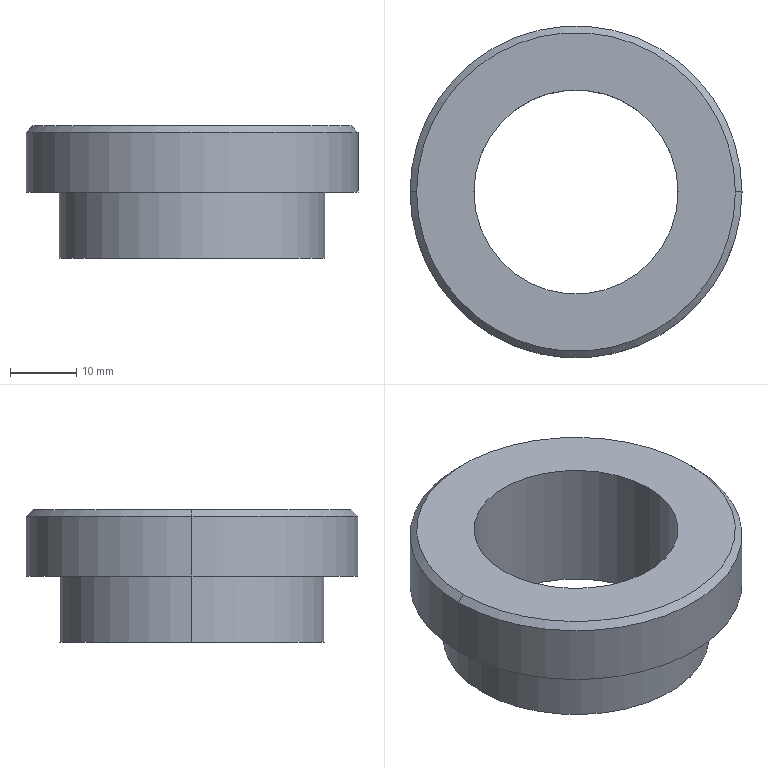Part | SolidWorks | features Chamfer 1, HoleWzd 1, Revolution 1 | 1 solid | 11 faces | box 50 x 50 x 20 mm | volume 17271 mm3 | cylinder 6 | plane 3 | cone 2 | commonest cylinder face diameters 30.75 x2 40 x2 50 x2
STEP:
#1=CARTESIAN_POINT('',(24.,0.,20.));
#2=VERTEX_POINT('',#1);
#3=CARTESIAN_POINT('',(-24.,0.,20.));
#4=VERTEX_POINT('',#3);
#5=CARTESIAN_POINT('',(0.,0.,20.));
#6=DIRECTION('',(0.,0.,1.));
#7=DIRECTION('',(-1.,0.,0.));
#8=AXIS2_PLACEMENT_3D('',#5,#6,#7);
#9=CIRCLE('',#8,24.);
#10=EDGE_CURVE('',#2,#4,#9,.T.);
#11=ORIENTED_EDGE('',*,*,#10,.F.);
#12=CARTESIAN_POINT('',(25.,0.,19.));
#13=VERTEX_POINT('',#12);
#14=CARTESIAN_POINT('',(24.,0.,20.));
#15=DIRECTION('',(0.7071,0.,-0.7071));
#16=VECTOR('',#15,1000.);
#17=LINE('',#14,#16);
#18=EDGE_CURVE('',#2,#13,#17,.T.);
#19=ORIENTED_EDGE('',*,*,#18,.T.);
#20=CARTESIAN_POINT('',(-25.,0.,19.));
#21=VERTEX_POINT('',#20);
#22=CARTESIAN_POINT('',(0.,0.,19.));
#23=DIRECTION('',(0.,0.,-1.));
#24=DIRECTION('',(-1.,0.,0.));
#25=AXIS2_PLACEMENT_3D('',#22,#23,#24);
#26=CIRCLE('',#25,25.);
#27=EDGE_CURVE('',#21,#13,#26,.T.);
#28=ORIENTED_EDGE('',*,*,#27,.F.);
#29=CARTESIAN_POINT('',(-24.,0.,20.));
#30=DIRECTION('',(-0.7071,0.,-0.7071));
#31=VECTOR('',#30,1000.);
#32=LINE('',#29,#31);
#33=EDGE_CURVE('',#4,#21,#32,.T.);
#34=ORIENTED_EDGE('',*,*,#33,.F.);
#35=EDGE_LOOP('',(#11,#19,#28,#34));
#36=FACE_OUTER_BOUND('',#35,.T.);
#37=CARTESIAN_POINT('',(0.,0.,20.));
#38=DIRECTION('',(0.,0.,-1.));
#39=DIRECTION('',(-1.,0.,0.));
#40=AXIS2_PLACEMENT_3D('',#37,#38,#39);
#41=CONICAL_SURFACE('',#40,24.,0.7854);
#42=ADVANCED_FACE('',(#36),#41,.T.);
#43=CARTESIAN_POINT('',(-15.375,0.,0.));
#44=VERTEX_POINT('',#43);
#45=CARTESIAN_POINT('',(15.375,0.,0.));
#46=VERTEX_POINT('',#45);
#47=CARTESIAN_POINT('',(0.,0.,0.));
#48=DIRECTION('',(0.,0.,1.));
#49=DIRECTION('',(1.,0.,0.));
#50=AXIS2_PLACEMENT_3D('',#47,#48,#49);
#51=CIRCLE('',#50,15.375);
#52=EDGE_CURVE('',#44,#46,#51,.T.);
#53=ORIENTED_EDGE('',*,*,#52,.F.);
#54=CARTESIAN_POINT('',(-15.375,0.,20.));
#55=VERTEX_POINT('',#54);
#56=CARTESIAN_POINT('',(-15.375,0.,20.));
#57=DIRECTION('',(0.,0.,1.));
#58=VECTOR('',#57,1000.);
#59=LINE('',#56,#58);
#60=EDGE_CURVE('',#44,#55,#59,.T.);
#61=ORIENTED_EDGE('',*,*,#60,.T.);
#62=CARTESIAN_POINT('',(15.375,0.,20.));
#63=VERTEX_POINT('',#62);
#64=CARTESIAN_POINT('',(0.,0.,20.));
#65=DIRECTION('',(0.,0.,1.));
#66=DIRECTION('',(1.,0.,0.));
#67=AXIS2_PLACEMENT_3D('',#64,#65,#66);
#68=CIRCLE('',#67,15.375);
#69=EDGE_CURVE('',#55,#63,#68,.T.);
#70=ORIENTED_EDGE('',*,*,#69,.T.);
#71=CARTESIAN_POINT('',(15.375,0.,20.));
#72=DIRECTION('',(0.,0.,1.));
#73=VECTOR('',#72,1000.);
#74=LINE('',#71,#73);
#75=EDGE_CURVE('',#46,#63,#74,.T.);
#76=ORIENTED_EDGE('',*,*,#75,.F.);
#77=EDGE_LOOP('',(#53,#61,#70,#76));
#78=FACE_OUTER_BOUND('',#77,.T.);
#79=CARTESIAN_POINT('',(0.,0.,20.));
#80=DIRECTION('',(0.,0.,1.));
#81=DIRECTION('',(1.,0.,0.));
#82=AXIS2_PLACEMENT_3D('',#79,#80,#81);
#83=CYLINDRICAL_SURFACE('',#82,15.375);
#84=ADVANCED_FACE('',(#78),#83,.F.);
#85=CARTESIAN_POINT('',(25.,0.,10.));
#86=VERTEX_POINT('',#85);
#87=CARTESIAN_POINT('',(-25.,0.,10.));
#88=VERTEX_POINT('',#87);
#89=CARTESIAN_POINT('',(0.,0.,10.));
#90=DIRECTION('',(0.,0.,1.));
#91=DIRECTION('',(1.,0.,0.));
#92=AXIS2_PLACEMENT_3D('',#89,#90,#91);
#93=CIRCLE('',#92,25.);
#94=EDGE_CURVE('',#86,#88,#93,.T.);
#95=ORIENTED_EDGE('',*,*,#94,.T.);
#96=CARTESIAN_POINT('',(-25.,0.,20.));
#97=DIRECTION('',(0.,0.,1.));
#98=VECTOR('',#97,1000.);
#99=LINE('',#96,#98);
#100=EDGE_CURVE('',#88,#21,#99,.T.);
#101=ORIENTED_EDGE('',*,*,#100,.T.);
#102=ORIENTED_EDGE('',*,*,#27,.T.);
#103=CARTESIAN_POINT('',(25.,0.,20.));
#104=DIRECTION('',(0.,0.,1.));
#105=VECTOR('',#104,1000.);
#106=LINE('',#103,#105);
#107=EDGE_CURVE('',#86,#13,#106,.T.);
#108=ORIENTED_EDGE('',*,*,#107,.F.);
#109=EDGE_LOOP('',(#95,#101,#102,#108));
#110=FACE_OUTER_BOUND('',#109,.T.);
#111=CARTESIAN_POINT('',(0.,0.,20.));
#112=DIRECTION('',(0.,0.,1.));
#113=DIRECTION('',(1.,0.,0.));
#114=AXIS2_PLACEMENT_3D('',#111,#112,#113);
#115=CYLINDRICAL_SURFACE('',#114,25.);
#116=ADVANCED_FACE('',(#110),#115,.T.);
#117=CARTESIAN_POINT('',(20.,0.,0.));
#118=VERTEX_POINT('',#117);
#119=CARTESIAN_POINT('',(-20.,0.,0.));
#120=VERTEX_POINT('',#119);
#121=CARTESIAN_POINT('',(0.,0.,0.));
#122=DIRECTION('',(0.,0.,1.));
#123=DIRECTION('',(1.,0.,0.));
#124=AXIS2_PLACEMENT_3D('',#121,#122,#123);
#125=CIRCLE('',#124,20.);
#126=EDGE_CURVE('',#118,#120,#125,.T.);
#127=ORIENTED_EDGE('',*,*,#126,.T.);
#128=CARTESIAN_POINT('',(-20.,0.,10.));
#129=VERTEX_POINT('',#128);
#130=CARTESIAN_POINT('',(-20.,0.,20.));
#131=DIRECTION('',(0.,0.,1.));
#132=VECTOR('',#131,1000.);
#133=LINE('',#130,#132);
#134=EDGE_CURVE('',#120,#129,#133,.T.);
#135=ORIENTED_EDGE('',*,*,#134,.T.);
#136=CARTESIAN_POINT('',(20.,0.,10.));
#137=VERTEX_POINT('',#136);
#138=CARTESIAN_POINT('',(0.,0.,10.));
#139=DIRECTION('',(0.,0.,1.));
#140=DIRECTION('',(1.,0.,0.));
#141=AXIS2_PLACEMENT_3D('',#138,#139,#140);
#142=CIRCLE('',#141,20.);
#143=EDGE_CURVE('',#137,#129,#142,.T.);
#144=ORIENTED_EDGE('',*,*,#143,.F.);
#145=CARTESIAN_POINT('',(20.,0.,20.));
#146=DIRECTION('',(0.,0.,1.));
#147=VECTOR('',#146,1000.);
#148=LINE('',#145,#147);
#149=EDGE_CURVE('',#118,#137,#148,.T.);
#150=ORIENTED_EDGE('',*,*,#149,.F.);
#151=EDGE_LOOP('',(#127,#135,#144,#150));
#152=FACE_OUTER_BOUND('',#151,.T.);
#153=CARTESIAN_POINT('',(0.,0.,20.));
#154=DIRECTION('',(0.,0.,1.));
#155=DIRECTION('',(1.,0.,0.));
#156=AXIS2_PLACEMENT_3D('',#153,#154,#155);
#157=CYLINDRICAL_SURFACE('',#156,20.);
#158=ADVANCED_FACE('',(#152),#157,.T.);
#159=CARTESIAN_POINT('',(0.,0.,0.));
#160=DIRECTION('',(0.,0.,1.));
#161=DIRECTION('',(1.,0.,0.));
#162=AXIS2_PLACEMENT_3D('',#159,#160,#161);
#163=CIRCLE('',#162,15.375);
#164=EDGE_CURVE('',#46,#44,#163,.T.);
#165=ORIENTED_EDGE('',*,*,#164,.T.);
#166=ORIENTED_EDGE('',*,*,#52,.T.);
#167=EDGE_LOOP('',(#165,#166));
#168=FACE_BOUND('',#167,.T.);
#169=ORIENTED_EDGE('',*,*,#126,.F.);
#170=CARTESIAN_POINT('',(0.,0.,0.));
#171=DIRECTION('',(0.,0.,1.));
#172=DIRECTION('',(1.,0.,0.));
#173=AXIS2_PLACEMENT_3D('',#170,#171,#172);
#174=CIRCLE('',#173,20.);
#175=EDGE_CURVE('',#120,#118,#174,.T.);
#176=ORIENTED_EDGE('',*,*,#175,.F.);
#177=EDGE_LOOP('',(#169,#176));
#178=FACE_OUTER_BOUND('',#177,.T.);
#179=CARTESIAN_POINT('',(0.,0.,0.));
#180=DIRECTION('',(0.,0.,1.));
#181=DIRECTION('',(1.,0.,0.));
#182=AXIS2_PLACEMENT_3D('',#179,#180,#181);
#183=PLANE('',#182);
#184=ADVANCED_FACE('',(#168,#178),#183,.F.);
#185=ORIENTED_EDGE('',*,*,#134,.F.);
#186=ORIENTED_EDGE('',*,*,#175,.T.);
#187=ORIENTED_EDGE('',*,*,#149,.T.);
#188=CARTESIAN_POINT('',(0.,0.,10.));
#189=DIRECTION('',(0.,0.,1.));
#190=DIRECTION('',(1.,0.,0.));
#191=AXIS2_PLACEMENT_3D('',#188,#189,#190);
#192=CIRCLE('',#191,20.);
#193=EDGE_CURVE('',#129,#137,#192,.T.);
#194=ORIENTED_EDGE('',*,*,#193,.F.);
#195=EDGE_LOOP('',(#185,#186,#187,#194));
#196=FACE_OUTER_BOUND('',#195,.T.);
#197=CARTESIAN_POINT('',(0.,0.,20.));
#198=DIRECTION('',(0.,0.,1.));
#199=DIRECTION('',(1.,0.,0.));
#200=AXIS2_PLACEMENT_3D('',#197,#198,#199);
#201=CYLINDRICAL_SURFACE('',#200,20.);
#202=ADVANCED_FACE('',(#196),#201,.T.);
#203=ORIENTED_EDGE('',*,*,#94,.F.);
#204=CARTESIAN_POINT('',(0.,0.,10.));
#205=DIRECTION('',(0.,0.,1.));
#206=DIRECTION('',(1.,0.,0.));
#207=AXIS2_PLACEMENT_3D('',#204,#205,#206);
#208=CIRCLE('',#207,25.);
#209=EDGE_CURVE('',#88,#86,#208,.T.);
#210=ORIENTED_EDGE('',*,*,#209,.F.);
#211=EDGE_LOOP('',(#203,#210));
#212=FACE_OUTER_BOUND('',#211,.T.);
#213=ORIENTED_EDGE('',*,*,#143,.T.);
#214=ORIENTED_EDGE('',*,*,#193,.T.);
#215=EDGE_LOOP('',(#213,#214));
#216=FACE_BOUND('',#215,.T.);
#217=CARTESIAN_POINT('',(0.,20.,10.));
#218=DIRECTION('',(0.,0.,1.));
#219=DIRECTION('',(1.,0.,0.));
#220=AXIS2_PLACEMENT_3D('',#217,#218,#219);
#221=PLANE('',#220);
#222=ADVANCED_FACE('',(#212,#216),#221,.F.);
#223=ORIENTED_EDGE('',*,*,#100,.F.);
#224=ORIENTED_EDGE('',*,*,#209,.T.);
#225=ORIENTED_EDGE('',*,*,#107,.T.);
#226=CARTESIAN_POINT('',(0.,0.,19.));
#227=DIRECTION('',(0.,0.,-1.));
#228=DIRECTION('',(-1.,0.,0.));
#229=AXIS2_PLACEMENT_3D('',#226,#227,#228);
#230=CIRCLE('',#229,25.);
#231=EDGE_CURVE('',#13,#21,#230,.T.);
#232=ORIENTED_EDGE('',*,*,#231,.T.);
#233=EDGE_LOOP('',(#223,#224,#225,#232));
#234=FACE_OUTER_BOUND('',#233,.T.);
#235=CARTESIAN_POINT('',(0.,0.,20.));
#236=DIRECTION('',(0.,0.,1.));
#237=DIRECTION('',(1.,0.,0.));
#238=AXIS2_PLACEMENT_3D('',#235,#236,#237);
#239=CYLINDRICAL_SURFACE('',#238,25.);
#240=ADVANCED_FACE('',(#234),#239,.T.);
#241=CARTESIAN_POINT('',(0.,0.,20.));
#242=DIRECTION('',(0.,0.,1.));
#243=DIRECTION('',(-1.,0.,0.));
#244=AXIS2_PLACEMENT_3D('',#241,#242,#243);
#245=CIRCLE('',#244,24.);
#246=EDGE_CURVE('',#4,#2,#245,.T.);
#247=ORIENTED_EDGE('',*,*,#246,.T.);
#248=ORIENTED_EDGE('',*,*,#10,.T.);
#249=EDGE_LOOP('',(#247,#248));
#250=FACE_OUTER_BOUND('',#249,.T.);
#251=CARTESIAN_POINT('',(0.,0.,20.));
#252=DIRECTION('',(0.,0.,1.));
#253=DIRECTION('',(1.,0.,0.));
#254=AXIS2_PLACEMENT_3D('',#251,#252,#253);
#255=CIRCLE('',#254,15.375);
#256=EDGE_CURVE('',#63,#55,#255,.T.);
#257=ORIENTED_EDGE('',*,*,#256,.F.);
#258=ORIENTED_EDGE('',*,*,#69,.F.);
#259=EDGE_LOOP('',(#257,#258));
#260=FACE_BOUND('',#259,.T.);
#261=CARTESIAN_POINT('',(0.,25.,20.));
#262=DIRECTION('',(0.,0.,-1.));
#263=DIRECTION('',(-1.,0.,0.));
#264=AXIS2_PLACEMENT_3D('',#261,#262,#263);
#265=PLANE('',#264);
#266=ADVANCED_FACE('',(#250,#260),#265,.F.);
#267=ORIENTED_EDGE('',*,*,#60,.F.);
#268=ORIENTED_EDGE('',*,*,#164,.F.);
#269=ORIENTED_EDGE('',*,*,#75,.T.);
#270=ORIENTED_EDGE('',*,*,#256,.T.);
#271=EDGE_LOOP('',(#267,#268,#269,#270));
#272=FACE_OUTER_BOUND('',#271,.T.);
#273=CARTESIAN_POINT('',(0.,0.,20.));
#274=DIRECTION('',(0.,0.,1.));
#275=DIRECTION('',(1.,0.,0.));
#276=AXIS2_PLACEMENT_3D('',#273,#274,#275);
#277=CYLINDRICAL_SURFACE('',#276,15.375);
#278=ADVANCED_FACE('',(#272),#277,.F.);
#279=ORIENTED_EDGE('',*,*,#18,.F.);
#280=ORIENTED_EDGE('',*,*,#246,.F.);
#281=ORIENTED_EDGE('',*,*,#33,.T.);
#282=ORIENTED_EDGE('',*,*,#231,.F.);
#283=EDGE_LOOP('',(#279,#280,#281,#282));
#284=FACE_OUTER_BOUND('',#283,.T.);
#285=CARTESIAN_POINT('',(0.,0.,20.));
#286=DIRECTION('',(0.,0.,-1.));
#287=DIRECTION('',(-1.,0.,0.));
#288=AXIS2_PLACEMENT_3D('',#285,#286,#287);
#289=CONICAL_SURFACE('',#288,24.,0.7854);
#290=ADVANCED_FACE('',(#284),#289,.T.);
#291=CLOSED_SHELL('',(#42,#84,#116,#158,#184,#202,#222,#240,#266,#278,#290));
#292=MANIFOLD_SOLID_BREP('',#291);
#293=CARTESIAN_POINT('',(0.,0.,0.));
#294=DIRECTION('',(0.,0.,1.));
#295=DIRECTION('',(1.,0.,0.));
#296=AXIS2_PLACEMENT_3D('',#293,#294,#295);
#297=(LENGTH_UNIT()NAMED_UNIT(*)SI_UNIT(.MILLI.,.METRE.));
#298=UNCERTAINTY_MEASURE_WITH_UNIT(LENGTH_MEASURE(0.00001),#297,'','');
#299=(NAMED_UNIT(*)PLANE_ANGLE_UNIT()SI_UNIT($,.RADIAN.));
#300=(NAMED_UNIT(*)SI_UNIT($,.STERADIAN.)SOLID_ANGLE_UNIT());
#301=(GEOMETRIC_REPRESENTATION_CONTEXT(3)GLOBAL_UNCERTAINTY_ASSIGNED_CONTEXT((#298))GLOBAL_UNIT_ASSIGNED_CONTEXT((#297,#299,#300))REPRESENTATION_CONTEXT('',''));
#302=ADVANCED_BREP_SHAPE_REPRESENTATION('',(#292,#296),#301);